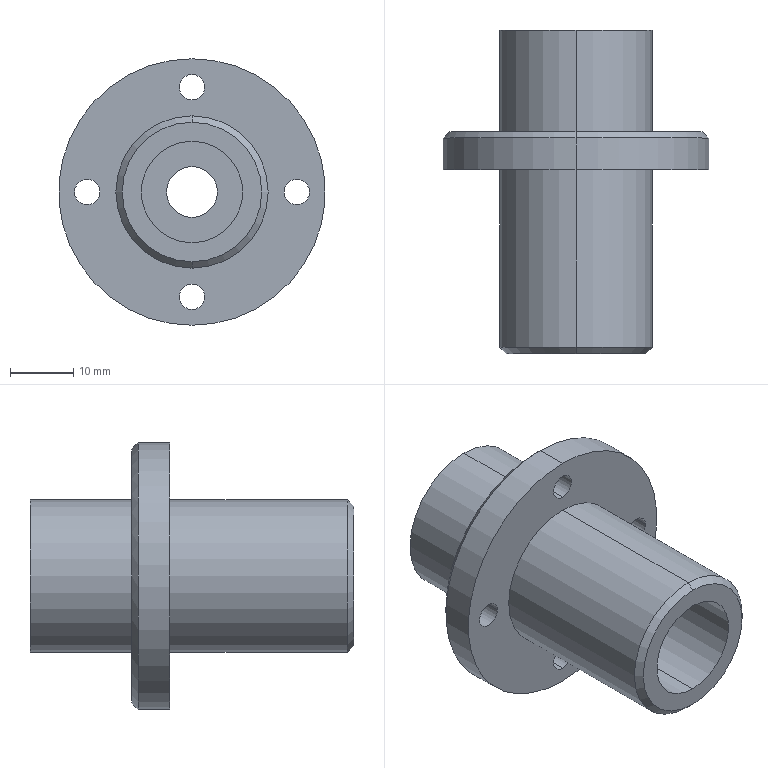Part | SolidWorks | features ICE 4, Chamfer 1, CirPattern 1, Extrusion 1 | 1 solid | 39 faces | box 42 x 51 x 42 mm | volume 18428 mm3 | cylinder 26 | plane 9 | cone 4 | commonest cylinder face diameters 4 x8 6 x8 24 x4 8 x2 16 x2 42 x2
STEP:
#1=CARTESIAN_POINT('',(0.,35.,20.));
#2=VERTEX_POINT('',#1);
#3=CARTESIAN_POINT('',(0.,35.,-20.));
#4=VERTEX_POINT('',#3);
#5=CARTESIAN_POINT('',(0.,35.,0.));
#6=DIRECTION('',(0.,1.,0.));
#7=DIRECTION('',(0.,0.,1.));
#8=AXIS2_PLACEMENT_3D('',#5,#6,#7);
#9=CIRCLE('',#8,20.);
#10=EDGE_CURVE('',#2,#4,#9,.T.);
#11=ORIENTED_EDGE('',*,*,#10,.F.);
#12=CARTESIAN_POINT('',(0.,34.,21.));
#13=VERTEX_POINT('',#12);
#14=CARTESIAN_POINT('',(0.,35.,20.));
#15=DIRECTION('',(0.,-0.7071,0.7071));
#16=VECTOR('',#15,1000.);
#17=LINE('',#14,#16);
#18=EDGE_CURVE('',#2,#13,#17,.T.);
#19=ORIENTED_EDGE('',*,*,#18,.T.);
#20=CARTESIAN_POINT('',(0.,34.,-21.));
#21=VERTEX_POINT('',#20);
#22=CARTESIAN_POINT('',(0.,34.,0.));
#23=DIRECTION('',(0.,-1.,0.));
#24=DIRECTION('',(0.,0.,1.));
#25=AXIS2_PLACEMENT_3D('',#22,#23,#24);
#26=CIRCLE('',#25,21.);
#27=EDGE_CURVE('',#21,#13,#26,.T.);
#28=ORIENTED_EDGE('',*,*,#27,.F.);
#29=CARTESIAN_POINT('',(0.,35.,-20.));
#30=DIRECTION('',(0.,-0.7071,-0.7071));
#31=VECTOR('',#30,1000.);
#32=LINE('',#29,#31);
#33=EDGE_CURVE('',#4,#21,#32,.T.);
#34=ORIENTED_EDGE('',*,*,#33,.F.);
#35=EDGE_LOOP('',(#11,#19,#28,#34));
#36=FACE_OUTER_BOUND('',#35,.T.);
#37=CARTESIAN_POINT('',(0.,35.,0.));
#38=DIRECTION('',(0.,-1.,0.));
#39=DIRECTION('',(0.,0.,-1.));
#40=AXIS2_PLACEMENT_3D('',#37,#38,#39);
#41=CONICAL_SURFACE('',#40,20.,0.7854);
#42=ADVANCED_FACE('',(#36),#41,.T.);
#43=CARTESIAN_POINT('',(0.,0.,-11.));
#44=VERTEX_POINT('',#43);
#45=CARTESIAN_POINT('',(0.,0.,11.));
#46=VERTEX_POINT('',#45);
#47=CARTESIAN_POINT('',(0.,0.,0.));
#48=DIRECTION('',(0.,-1.,0.));
#49=DIRECTION('',(0.,0.,1.));
#50=AXIS2_PLACEMENT_3D('',#47,#48,#49);
#51=CIRCLE('',#50,11.);
#52=EDGE_CURVE('',#44,#46,#51,.T.);
#53=ORIENTED_EDGE('',*,*,#52,.F.);
#54=CARTESIAN_POINT('',(0.,1.,-12.));
#55=VERTEX_POINT('',#54);
#56=CARTESIAN_POINT('',(0.,1.,-12.));
#57=DIRECTION('',(0.,0.7071,-0.7071));
#58=VECTOR('',#57,1000.);
#59=LINE('',#56,#58);
#60=EDGE_CURVE('',#44,#55,#59,.T.);
#61=ORIENTED_EDGE('',*,*,#60,.T.);
#62=CARTESIAN_POINT('',(0.,1.,12.));
#63=VERTEX_POINT('',#62);
#64=CARTESIAN_POINT('',(0.,1.,0.));
#65=DIRECTION('',(0.,1.,0.));
#66=DIRECTION('',(0.,0.,1.));
#67=AXIS2_PLACEMENT_3D('',#64,#65,#66);
#68=CIRCLE('',#67,12.);
#69=EDGE_CURVE('',#63,#55,#68,.T.);
#70=ORIENTED_EDGE('',*,*,#69,.F.);
#71=CARTESIAN_POINT('',(0.,1.,12.));
#72=DIRECTION('',(0.,0.7071,0.7071));
#73=VECTOR('',#72,1000.);
#74=LINE('',#71,#73);
#75=EDGE_CURVE('',#46,#63,#74,.T.);
#76=ORIENTED_EDGE('',*,*,#75,.F.);
#77=EDGE_LOOP('',(#53,#61,#70,#76));
#78=FACE_OUTER_BOUND('',#77,.T.);
#79=CARTESIAN_POINT('',(0.,1.,0.));
#80=DIRECTION('',(0.,1.,0.));
#81=DIRECTION('',(0.,0.,1.));
#82=AXIS2_PLACEMENT_3D('',#79,#80,#81);
#83=CONICAL_SURFACE('',#82,12.,0.7854);
#84=ADVANCED_FACE('',(#78),#83,.T.);
#85=CARTESIAN_POINT('',(-19.5,32.,0.));
#86=VERTEX_POINT('',#85);
#87=CARTESIAN_POINT('',(-13.5,32.,0.));
#88=VERTEX_POINT('',#87);
#89=CARTESIAN_POINT('',(-16.5,32.,0.));
#90=DIRECTION('',(0.,1.,0.));
#91=DIRECTION('',(1.,0.,0.));
#92=AXIS2_PLACEMENT_3D('',#89,#90,#91);
#93=CIRCLE('',#92,3.);
#94=EDGE_CURVE('',#86,#88,#93,.T.);
#95=ORIENTED_EDGE('',*,*,#94,.F.);
#96=CARTESIAN_POINT('',(-19.5,35.,0.));
#97=VERTEX_POINT('',#96);
#98=CARTESIAN_POINT('',(-19.5,32.,0.));
#99=DIRECTION('',(0.,1.,0.));
#100=VECTOR('',#99,1000.);
#101=LINE('',#98,#100);
#102=EDGE_CURVE('',#86,#97,#101,.T.);
#103=ORIENTED_EDGE('',*,*,#102,.T.);
#104=CARTESIAN_POINT('',(-13.5,35.,0.));
#105=VERTEX_POINT('',#104);
#106=CARTESIAN_POINT('',(-16.5,35.,0.));
#107=DIRECTION('',(0.,1.,0.));
#108=DIRECTION('',(1.,0.,0.));
#109=AXIS2_PLACEMENT_3D('',#106,#107,#108);
#110=CIRCLE('',#109,3.);
#111=EDGE_CURVE('',#97,#105,#110,.T.);
#112=ORIENTED_EDGE('',*,*,#111,.T.);
#113=CARTESIAN_POINT('',(-13.5,32.,0.));
#114=DIRECTION('',(0.,1.,0.));
#115=VECTOR('',#114,1000.);
#116=LINE('',#113,#115);
#117=EDGE_CURVE('',#88,#105,#116,.T.);
#118=ORIENTED_EDGE('',*,*,#117,.F.);
#119=EDGE_LOOP('',(#95,#103,#112,#118));
#120=FACE_OUTER_BOUND('',#119,.T.);
#121=CARTESIAN_POINT('',(-16.5,32.,0.));
#122=DIRECTION('',(0.,1.,0.));
#123=DIRECTION('',(1.,0.,0.));
#124=AXIS2_PLACEMENT_3D('',#121,#122,#123);
#125=CYLINDRICAL_SURFACE('',#124,3.);
#126=ADVANCED_FACE('',(#120),#125,.F.);
#127=CARTESIAN_POINT('',(0.,32.,19.5));
#128=VERTEX_POINT('',#127);
#129=CARTESIAN_POINT('',(0.,32.,13.5));
#130=VERTEX_POINT('',#129);
#131=CARTESIAN_POINT('',(0.,32.,16.5));
#132=DIRECTION('',(0.,1.,0.));
#133=DIRECTION('',(0.,0.,-1.));
#134=AXIS2_PLACEMENT_3D('',#131,#132,#133);
#135=CIRCLE('',#134,3.);
#136=EDGE_CURVE('',#128,#130,#135,.T.);
#137=ORIENTED_EDGE('',*,*,#136,.F.);
#138=CARTESIAN_POINT('',(0.,35.,19.5));
#139=VERTEX_POINT('',#138);
#140=CARTESIAN_POINT('',(0.,32.,19.5));
#141=DIRECTION('',(0.,1.,0.));
#142=VECTOR('',#141,1000.);
#143=LINE('',#140,#142);
#144=EDGE_CURVE('',#128,#139,#143,.T.);
#145=ORIENTED_EDGE('',*,*,#144,.T.);
#146=CARTESIAN_POINT('',(0.,35.,13.5));
#147=VERTEX_POINT('',#146);
#148=CARTESIAN_POINT('',(0.,35.,16.5));
#149=DIRECTION('',(0.,1.,0.));
#150=DIRECTION('',(0.,0.,-1.));
#151=AXIS2_PLACEMENT_3D('',#148,#149,#150);
#152=CIRCLE('',#151,3.);
#153=EDGE_CURVE('',#139,#147,#152,.T.);
#154=ORIENTED_EDGE('',*,*,#153,.T.);
#155=CARTESIAN_POINT('',(0.,32.,13.5));
#156=DIRECTION('',(0.,1.,0.));
#157=VECTOR('',#156,1000.);
#158=LINE('',#155,#157);
#159=EDGE_CURVE('',#130,#147,#158,.T.);
#160=ORIENTED_EDGE('',*,*,#159,.F.);
#161=EDGE_LOOP('',(#137,#145,#154,#160));
#162=FACE_OUTER_BOUND('',#161,.T.);
#163=CARTESIAN_POINT('',(0.,32.,16.5));
#164=DIRECTION('',(0.,1.,0.));
#165=DIRECTION('',(0.,0.,-1.));
#166=AXIS2_PLACEMENT_3D('',#163,#164,#165);
#167=CYLINDRICAL_SURFACE('',#166,3.);
#168=ADVANCED_FACE('',(#162),#167,.F.);
#169=CARTESIAN_POINT('',(19.5,32.,0.));
#170=VERTEX_POINT('',#169);
#171=CARTESIAN_POINT('',(13.5,32.,0.));
#172=VERTEX_POINT('',#171);
#173=CARTESIAN_POINT('',(16.5,32.,0.));
#174=DIRECTION('',(0.,1.,0.));
#175=DIRECTION('',(-1.,0.,0.));
#176=AXIS2_PLACEMENT_3D('',#173,#174,#175);
#177=CIRCLE('',#176,3.);
#178=EDGE_CURVE('',#170,#172,#177,.T.);
#179=ORIENTED_EDGE('',*,*,#178,.F.);
#180=CARTESIAN_POINT('',(19.5,35.,0.));
#181=VERTEX_POINT('',#180);
#182=CARTESIAN_POINT('',(19.5,32.,0.));
#183=DIRECTION('',(0.,1.,0.));
#184=VECTOR('',#183,1000.);
#185=LINE('',#182,#184);
#186=EDGE_CURVE('',#170,#181,#185,.T.);
#187=ORIENTED_EDGE('',*,*,#186,.T.);
#188=CARTESIAN_POINT('',(13.5,35.,0.));
#189=VERTEX_POINT('',#188);
#190=CARTESIAN_POINT('',(16.5,35.,0.));
#191=DIRECTION('',(0.,1.,0.));
#192=DIRECTION('',(-1.,0.,0.));
#193=AXIS2_PLACEMENT_3D('',#190,#191,#192);
#194=CIRCLE('',#193,3.);
#195=EDGE_CURVE('',#181,#189,#194,.T.);
#196=ORIENTED_EDGE('',*,*,#195,.T.);
#197=CARTESIAN_POINT('',(13.5,32.,0.));
#198=DIRECTION('',(0.,1.,0.));
#199=VECTOR('',#198,1000.);
#200=LINE('',#197,#199);
#201=EDGE_CURVE('',#172,#189,#200,.T.);
#202=ORIENTED_EDGE('',*,*,#201,.F.);
#203=EDGE_LOOP('',(#179,#187,#196,#202));
#204=FACE_OUTER_BOUND('',#203,.T.);
#205=CARTESIAN_POINT('',(16.5,32.,0.));
#206=DIRECTION('',(0.,1.,0.));
#207=DIRECTION('',(-1.,0.,0.));
#208=AXIS2_PLACEMENT_3D('',#205,#206,#207);
#209=CYLINDRICAL_SURFACE('',#208,3.);
#210=ADVANCED_FACE('',(#204),#209,.F.);
#211=CARTESIAN_POINT('',(-18.5,29.,0.));
#212=VERTEX_POINT('',#211);
#213=CARTESIAN_POINT('',(-14.5,29.,0.));
#214=VERTEX_POINT('',#213);
#215=CARTESIAN_POINT('',(-16.5,29.,0.));
#216=DIRECTION('',(0.,1.,0.));
#217=DIRECTION('',(1.,0.,0.));
#218=AXIS2_PLACEMENT_3D('',#215,#216,#217);
#219=CIRCLE('',#218,2.);
#220=EDGE_CURVE('',#212,#214,#219,.T.);
#221=ORIENTED_EDGE('',*,*,#220,.F.);
#222=CARTESIAN_POINT('',(-18.5,32.,0.));
#223=VERTEX_POINT('',#222);
#224=CARTESIAN_POINT('',(-18.5,29.,0.));
#225=DIRECTION('',(0.,1.,0.));
#226=VECTOR('',#225,1000.);
#227=LINE('',#224,#226);
#228=EDGE_CURVE('',#212,#223,#227,.T.);
#229=ORIENTED_EDGE('',*,*,#228,.T.);
#230=CARTESIAN_POINT('',(-14.5,32.,0.));
#231=VERTEX_POINT('',#230);
#232=CARTESIAN_POINT('',(-16.5,32.,0.));
#233=DIRECTION('',(0.,-1.,0.));
#234=DIRECTION('',(0.,0.,1.));
#235=AXIS2_PLACEMENT_3D('',#232,#233,#234);
#236=CIRCLE('',#235,2.);
#237=EDGE_CURVE('',#231,#223,#236,.T.);
#238=ORIENTED_EDGE('',*,*,#237,.F.);
#239=CARTESIAN_POINT('',(-14.5,29.,0.));
#240=DIRECTION('',(0.,1.,0.));
#241=VECTOR('',#240,1000.);
#242=LINE('',#239,#241);
#243=EDGE_CURVE('',#214,#231,#242,.T.);
#244=ORIENTED_EDGE('',*,*,#243,.F.);
#245=EDGE_LOOP('',(#221,#229,#238,#244));
#246=FACE_OUTER_BOUND('',#245,.T.);
#247=CARTESIAN_POINT('',(-16.5,29.,0.));
#248=DIRECTION('',(0.,1.,0.));
#249=DIRECTION('',(1.,0.,0.));
#250=AXIS2_PLACEMENT_3D('',#247,#248,#249);
#251=CYLINDRICAL_SURFACE('',#250,2.);
#252=ADVANCED_FACE('',(#246),#251,.F.);
#253=CARTESIAN_POINT('',(0.,29.,18.5));
#254=VERTEX_POINT('',#253);
#255=CARTESIAN_POINT('',(0.,29.,14.5));
#256=VERTEX_POINT('',#255);
#257=CARTESIAN_POINT('',(0.,29.,16.5));
#258=DIRECTION('',(0.,1.,0.));
#259=DIRECTION('',(0.,0.,-1.));
#260=AXIS2_PLACEMENT_3D('',#257,#258,#259);
#261=CIRCLE('',#260,2.);
#262=EDGE_CURVE('',#254,#256,#261,.T.);
#263=ORIENTED_EDGE('',*,*,#262,.F.);
#264=CARTESIAN_POINT('',(0.,32.,18.5));
#265=VERTEX_POINT('',#264);
#266=CARTESIAN_POINT('',(0.,29.,18.5));
#267=DIRECTION('',(0.,1.,0.));
#268=VECTOR('',#267,1000.);
#269=LINE('',#266,#268);
#270=EDGE_CURVE('',#254,#265,#269,.T.);
#271=ORIENTED_EDGE('',*,*,#270,.T.);
#272=CARTESIAN_POINT('',(0.,32.,14.5));
#273=VERTEX_POINT('',#272);
#274=CARTESIAN_POINT('',(0.,32.,16.5));
#275=DIRECTION('',(0.,-1.,0.));
#276=DIRECTION('',(0.,0.,1.));
#277=AXIS2_PLACEMENT_3D('',#274,#275,#276);
#278=CIRCLE('',#277,2.);
#279=EDGE_CURVE('',#273,#265,#278,.T.);
#280=ORIENTED_EDGE('',*,*,#279,.F.);
#281=CARTESIAN_POINT('',(0.,29.,14.5));
#282=DIRECTION('',(0.,1.,0.));
#283=VECTOR('',#282,1000.);
#284=LINE('',#281,#283);
#285=EDGE_CURVE('',#256,#273,#284,.T.);
#286=ORIENTED_EDGE('',*,*,#285,.F.);
#287=EDGE_LOOP('',(#263,#271,#280,#286));
#288=FACE_OUTER_BOUND('',#287,.T.);
#289=CARTESIAN_POINT('',(0.,29.,16.5));
#290=DIRECTION('',(0.,1.,0.));
#291=DIRECTION('',(0.,0.,-1.));
#292=AXIS2_PLACEMENT_3D('',#289,#290,#291);
#293=CYLINDRICAL_SURFACE('',#292,2.);
#294=ADVANCED_FACE('',(#288),#293,.F.);
#295=CARTESIAN_POINT('',(18.5,29.,0.));
#296=VERTEX_POINT('',#295);
#297=CARTESIAN_POINT('',(14.5,29.,0.));
#298=VERTEX_POINT('',#297);
#299=CARTESIAN_POINT('',(16.5,29.,0.));
#300=DIRECTION('',(0.,1.,0.));
#301=DIRECTION('',(-1.,0.,0.));
#302=AXIS2_PLACEMENT_3D('',#299,#300,#301);
#303=CIRCLE('',#302,2.);
#304=EDGE_CURVE('',#296,#298,#303,.T.);
#305=ORIENTED_EDGE('',*,*,#304,.F.);
#306=CARTESIAN_POINT('',(18.5,32.,0.));
#307=VERTEX_POINT('',#306);
#308=CARTESIAN_POINT('',(18.5,29.,0.));
#309=DIRECTION('',(0.,1.,0.));
#310=VECTOR('',#309,1000.);
#311=LINE('',#308,#310);
#312=EDGE_CURVE('',#296,#307,#311,.T.);
#313=ORIENTED_EDGE('',*,*,#312,.T.);
#314=CARTESIAN_POINT('',(14.5,32.,0.));
#315=VERTEX_POINT('',#314);
#316=CARTESIAN_POINT('',(16.5,32.,0.));
#317=DIRECTION('',(0.,-1.,0.));
#318=DIRECTION('',(0.,0.,1.));
#319=AXIS2_PLACEMENT_3D('',#316,#317,#318);
#320=CIRCLE('',#319,2.);
#321=EDGE_CURVE('',#315,#307,#320,.T.);
#322=ORIENTED_EDGE('',*,*,#321,.F.);
#323=CARTESIAN_POINT('',(14.5,29.,0.));
#324=DIRECTION('',(0.,1.,0.));
#325=VECTOR('',#324,1000.);
#326=LINE('',#323,#325);
#327=EDGE_CURVE('',#298,#315,#326,.T.);
#328=ORIENTED_EDGE('',*,*,#327,.F.);
#329=EDGE_LOOP('',(#305,#313,#322,#328));
#330=FACE_OUTER_BOUND('',#329,.T.);
#331=CARTESIAN_POINT('',(16.5,29.,0.));
#332=DIRECTION('',(0.,1.,0.));
#333=DIRECTION('',(-1.,0.,0.));
#334=AXIS2_PLACEMENT_3D('',#331,#332,#333);
#335=CYLINDRICAL_SURFACE('',#334,2.);
#336=ADVANCED_FACE('',(#330),#335,.F.);
#337=CARTESIAN_POINT('',(0.,32.,-19.5));
#338=VERTEX_POINT('',#337);
#339=CARTESIAN_POINT('',(0.,32.,-13.5));
#340=VERTEX_POINT('',#339);
#341=CARTESIAN_POINT('',(0.,32.,-16.5));
#342=DIRECTION('',(0.,1.,0.));
#343=DIRECTION('',(0.,0.,1.));
#344=AXIS2_PLACEMENT_3D('',#341,#342,#343);
#345=CIRCLE('',#344,3.);
#346=EDGE_CURVE('',#338,#340,#345,.T.);
#347=ORIENTED_EDGE('',*,*,#346,.F.);
#348=CARTESIAN_POINT('',(0.,35.,-19.5));
#349=VERTEX_POINT('',#348);
#350=CARTESIAN_POINT('',(0.,32.,-19.5));
#351=DIRECTION('',(0.,1.,0.));
#352=VECTOR('',#351,1000.);
#353=LINE('',#350,#352);
#354=EDGE_CURVE('',#338,#349,#353,.T.);
#355=ORIENTED_EDGE('',*,*,#354,.T.);
#356=CARTESIAN_POINT('',(0.,35.,-13.5));
#357=VERTEX_POINT('',#356);
#358=CARTESIAN_POINT('',(0.,35.,-16.5));
#359=DIRECTION('',(0.,1.,0.));
#360=DIRECTION('',(0.,0.,1.));
#361=AXIS2_PLACEMENT_3D('',#358,#359,#360);
#362=CIRCLE('',#361,3.);
#363=EDGE_CURVE('',#349,#357,#362,.T.);
#364=ORIENTED_EDGE('',*,*,#363,.T.);
#365=CARTESIAN_POINT('',(0.,32.,-13.5));
#366=DIRECTION('',(0.,1.,0.));
#367=VECTOR('',#366,1000.);
#368=LINE('',#365,#367);
#369=EDGE_CURVE('',#340,#357,#368,.T.);
#370=ORIENTED_EDGE('',*,*,#369,.F.);
#371=EDGE_LOOP('',(#347,#355,#364,#370));
#372=FACE_OUTER_BOUND('',#371,.T.);
#373=CARTESIAN_POINT('',(0.,32.,-16.5));
#374=DIRECTION('',(0.,1.,0.));
#375=DIRECTION('',(0.,0.,1.));
#376=AXIS2_PLACEMENT_3D('',#373,#374,#375);
#377=CYLINDRICAL_SURFACE('',#376,3.);
#378=ADVANCED_FACE('',(#372),#377,.F.);
#379=CARTESIAN_POINT('',(0.,29.,21.));
#380=VERTEX_POINT('',#379);
#381=CARTESIAN_POINT('',(0.,29.,-21.));
#382=VERTEX_POINT('',#381);
#383=CARTESIAN_POINT('',(0.,29.,0.));
#384=DIRECTION('',(0.,1.,0.));
#385=DIRECTION('',(0.,0.,1.));
#386=AXIS2_PLACEMENT_3D('',#383,#384,#385);
#387=CIRCLE('',#386,21.);
#388=EDGE_CURVE('',#380,#382,#387,.T.);
#389=ORIENTED_EDGE('',*,*,#388,.T.);
#390=CARTESIAN_POINT('',(0.,29.,-21.));
#391=DIRECTION('',(0.,1.,0.));
#392=VECTOR('',#391,1000.);
#393=LINE('',#390,#392);
#394=EDGE_CURVE('',#382,#21,#393,.T.);
#395=ORIENTED_EDGE('',*,*,#394,.T.);
#396=ORIENTED_EDGE('',*,*,#27,.T.);
#397=CARTESIAN_POINT('',(0.,29.,21.));
#398=DIRECTION('',(0.,1.,0.));
#399=VECTOR('',#398,1000.);
#400=LINE('',#397,#399);
#401=EDGE_CURVE('',#380,#13,#400,.T.);
#402=ORIENTED_EDGE('',*,*,#401,.F.);
#403=EDGE_LOOP('',(#389,#395,#396,#402));
#404=FACE_OUTER_BOUND('',#403,.T.);
#405=CARTESIAN_POINT('',(0.,29.,0.));
#406=DIRECTION('',(0.,1.,0.));
#407=DIRECTION('',(0.,0.,1.));
#408=AXIS2_PLACEMENT_3D('',#405,#406,#407);
#409=CYLINDRICAL_SURFACE('',#408,21.);
#410=ADVANCED_FACE('',(#404),#409,.T.);
#411=CARTESIAN_POINT('',(0.,47.,8.));
#412=VERTEX_POINT('',#411);
#413=CARTESIAN_POINT('',(0.,47.,-8.));
#414=VERTEX_POINT('',#413);
#415=CARTESIAN_POINT('',(0.,47.,0.));
#416=DIRECTION('',(0.,-1.,0.));
#417=DIRECTION('',(0.,0.,-1.));
#418=AXIS2_PLACEMENT_3D('',#415,#416,#417);
#419=CIRCLE('',#418,8.);
#420=EDGE_CURVE('',#412,#414,#419,.T.);
#421=ORIENTED_EDGE('',*,*,#420,.F.);
#422=CARTESIAN_POINT('',(0.,0.,8.));
#423=VERTEX_POINT('',#422);
#424=CARTESIAN_POINT('',(0.,47.,8.));
#425=DIRECTION('',(0.,-1.,0.));
#426=VECTOR('',#425,1000.);
#427=LINE('',#424,#426);
#428=EDGE_CURVE('',#412,#423,#427,.T.);
#429=ORIENTED_EDGE('',*,*,#428,.T.);
#430=CARTESIAN_POINT('',(0.,0.,-8.));
#431=VERTEX_POINT('',#430);
#432=CARTESIAN_POINT('',(0.,0.,0.));
#433=DIRECTION('',(0.,-1.,0.));
#434=DIRECTION('',(0.,0.,-1.));
#435=AXIS2_PLACEMENT_3D('',#432,#433,#434);
#436=CIRCLE('',#435,8.);
#437=EDGE_CURVE('',#423,#431,#436,.T.);
#438=ORIENTED_EDGE('',*,*,#437,.T.);
#439=CARTESIAN_POINT('',(0.,47.,-8.));
#440=DIRECTION('',(0.,-1.,0.));
#441=VECTOR('',#440,1000.);
#442=LINE('',#439,#441);
#443=EDGE_CURVE('',#414,#431,#442,.T.);
#444=ORIENTED_EDGE('',*,*,#443,.F.);
#445=EDGE_LOOP('',(#421,#429,#438,#444));
#446=FACE_OUTER_BOUND('',#445,.T.);
#447=CARTESIAN_POINT('',(0.,47.,0.));
#448=DIRECTION('',(0.,-1.,0.));
#449=DIRECTION('',(0.,0.,-1.));
#450=AXIS2_PLACEMENT_3D('',#447,#448,#449);
#451=CYLINDRICAL_SURFACE('',#450,8.);
#452=ADVANCED_FACE('',(#446),#451,.F.);
#453=CARTESIAN_POINT('',(0.,51.,12.));
#454=VERTEX_POINT('',#453);
#455=CARTESIAN_POINT('',(0.,51.,-12.));
#456=VERTEX_POINT('',#455);
#457=CARTESIAN_POINT('',(0.,51.,0.));
#458=DIRECTION('',(0.,1.,0.));
#459=DIRECTION('',(0.,0.,1.));
#460=AXIS2_PLACEMENT_3D('',#457,#458,#459);
#461=CIRCLE('',#460,12.);
#462=EDGE_CURVE('',#454,#456,#461,.T.);
#463=ORIENTED_EDGE('',*,*,#462,.F.);
#464=CARTESIAN_POINT('',(0.,35.,12.));
#465=VERTEX_POINT('',#464);
#466=CARTESIAN_POINT('',(0.,51.,12.));
#467=DIRECTION('',(0.,-1.,0.));
#468=VECTOR('',#467,1000.);
#469=LINE('',#466,#468);
#470=EDGE_CURVE('',#454,#465,#469,.T.);
#471=ORIENTED_EDGE('',*,*,#470,.T.);
#472=CARTESIAN_POINT('',(0.,35.,-12.));
#473=VERTEX_POINT('',#472);
#474=CARTESIAN_POINT('',(0.,35.,0.));
#475=DIRECTION('',(0.,1.,0.));
#476=DIRECTION('',(0.,0.,1.));
#477=AXIS2_PLACEMENT_3D('',#474,#475,#476);
#478=CIRCLE('',#477,12.);
#479=EDGE_CURVE('',#465,#473,#478,.T.);
#480=ORIENTED_EDGE('',*,*,#479,.T.);
#481=CARTESIAN_POINT('',(0.,51.,-12.));
#482=DIRECTION('',(0.,-1.,0.));
#483=VECTOR('',#482,1000.);
#484=LINE('',#481,#483);
#485=EDGE_CURVE('',#456,#473,#484,.T.);
#486=ORIENTED_EDGE('',*,*,#485,.F.);
#487=EDGE_LOOP('',(#463,#471,#480,#486));
#488=FACE_OUTER_BOUND('',#487,.T.);
#489=CARTESIAN_POINT('',(0.,51.,0.));
#490=DIRECTION('',(0.,-1.,0.));
#491=DIRECTION('',(0.,0.,-1.));
#492=AXIS2_PLACEMENT_3D('',#489,#490,#491);
#493=CYLINDRICAL_SURFACE('',#492,12.);
#494=ADVANCED_FACE('',(#488),#493,.T.);
#495=CARTESIAN_POINT('',(0.,51.,-4.));
#496=VERTEX_POINT('',#495);
#497=CARTESIAN_POINT('',(0.,51.,4.));
#498=VERTEX_POINT('',#497);
#499=CARTESIAN_POINT('',(0.,51.,0.));
#500=DIRECTION('',(0.,1.,0.));
#501=DIRECTION('',(0.,0.,1.));
#502=AXIS2_PLACEMENT_3D('',#499,#500,#501);
#503=CIRCLE('',#502,4.);
#504=EDGE_CURVE('',#496,#498,#503,.T.);
#505=ORIENTED_EDGE('',*,*,#504,.T.);
#506=CARTESIAN_POINT('',(0.,47.,4.));
#507=VERTEX_POINT('',#506);
#508=CARTESIAN_POINT('',(0.,51.,4.));
#509=DIRECTION('',(0.,-1.,0.));
#510=VECTOR('',#509,1000.);
#511=LINE('',#508,#510);
#512=EDGE_CURVE('',#498,#507,#511,.T.);
#513=ORIENTED_EDGE('',*,*,#512,.T.);
#514=CARTESIAN_POINT('',(0.,47.,-4.));
#515=VERTEX_POINT('',#514);
#516=CARTESIAN_POINT('',(0.,47.,0.));
#517=DIRECTION('',(0.,-1.,0.));
#518=DIRECTION('',(0.,0.,-1.));
#519=AXIS2_PLACEMENT_3D('',#516,#517,#518);
#520=CIRCLE('',#519,4.);
#521=EDGE_CURVE('',#507,#515,#520,.T.);
#522=ORIENTED_EDGE('',*,*,#521,.T.);
#523=CARTESIAN_POINT('',(0.,51.,-4.));
#524=DIRECTION('',(0.,-1.,0.));
#525=VECTOR('',#524,1000.);
#526=LINE('',#523,#525);
#527=EDGE_CURVE('',#496,#515,#526,.T.);
#528=ORIENTED_EDGE('',*,*,#527,.F.);
#529=EDGE_LOOP('',(#505,#513,#522,#528));
#530=FACE_OUTER_BOUND('',#529,.T.);
#531=CARTESIAN_POINT('',(0.,51.,0.));
#532=DIRECTION('',(0.,-1.,0.));
#533=DIRECTION('',(0.,0.,-1.));
#534=AXIS2_PLACEMENT_3D('',#531,#532,#533);
#535=CYLINDRICAL_SURFACE('',#534,4.);
#536=ADVANCED_FACE('',(#530),#535,.F.);
#537=CARTESIAN_POINT('',(0.,29.,12.));
#538=VERTEX_POINT('',#537);
#539=CARTESIAN_POINT('',(0.,29.,-12.));
#540=VERTEX_POINT('',#539);
#541=CARTESIAN_POINT('',(0.,29.,0.));
#542=DIRECTION('',(0.,1.,0.));
#543=DIRECTION('',(0.,0.,1.));
#544=AXIS2_PLACEMENT_3D('',#541,#542,#543);
#545=CIRCLE('',#544,12.);
#546=EDGE_CURVE('',#538,#540,#545,.T.);
#547=ORIENTED_EDGE('',*,*,#546,.F.);
#548=CARTESIAN_POINT('',(0.,51.,12.));
#549=DIRECTION('',(0.,-1.,0.));
#550=VECTOR('',#549,1000.);
#551=LINE('',#548,#550);
#552=EDGE_CURVE('',#538,#63,#551,.T.);
#553=ORIENTED_EDGE('',*,*,#552,.T.);
#554=ORIENTED_EDGE('',*,*,#69,.T.);
#555=CARTESIAN_POINT('',(0.,51.,-12.));
#556=DIRECTION('',(0.,-1.,0.));
#557=VECTOR('',#556,1000.);
#558=LINE('',#555,#557);
#559=EDGE_CURVE('',#540,#55,#558,.T.);
#560=ORIENTED_EDGE('',*,*,#559,.F.);
#561=EDGE_LOOP('',(#547,#553,#554,#560));
#562=FACE_OUTER_BOUND('',#561,.T.);
#563=CARTESIAN_POINT('',(0.,51.,0.));
#564=DIRECTION('',(0.,-1.,0.));
#565=DIRECTION('',(0.,0.,-1.));
#566=AXIS2_PLACEMENT_3D('',#563,#564,#565);
#567=CYLINDRICAL_SURFACE('',#566,12.);
#568=ADVANCED_FACE('',(#562),#567,.T.);
#569=CARTESIAN_POINT('',(0.,29.,-18.5));
#570=VERTEX_POINT('',#569);
#571=CARTESIAN_POINT('',(0.,29.,-14.5));
#572=VERTEX_POINT('',#571);
#573=CARTESIAN_POINT('',(0.,29.,-16.5));
#574=DIRECTION('',(0.,1.,0.));
#575=DIRECTION('',(0.,0.,1.));
#576=AXIS2_PLACEMENT_3D('',#573,#574,#575);
#577=CIRCLE('',#576,2.);
#578=EDGE_CURVE('',#570,#572,#577,.T.);
#579=ORIENTED_EDGE('',*,*,#578,.F.);
#580=CARTESIAN_POINT('',(0.,32.,-18.5));
#581=VERTEX_POINT('',#580);
#582=CARTESIAN_POINT('',(0.,29.,-18.5));
#583=DIRECTION('',(0.,1.,0.));
#584=VECTOR('',#583,1000.);
#585=LINE('',#582,#584);
#586=EDGE_CURVE('',#570,#581,#585,.T.);
#587=ORIENTED_EDGE('',*,*,#586,.T.);
#588=CARTESIAN_POINT('',(0.,32.,-14.5));
#589=VERTEX_POINT('',#588);
#590=CARTESIAN_POINT('',(0.,32.,-16.5));
#591=DIRECTION('',(0.,-1.,0.));
#592=DIRECTION('',(0.,0.,1.));
#593=AXIS2_PLACEMENT_3D('',#590,#591,#592);
#594=CIRCLE('',#593,2.);
#595=EDGE_CURVE('',#589,#581,#594,.T.);
#596=ORIENTED_EDGE('',*,*,#595,.F.);
#597=CARTESIAN_POINT('',(0.,29.,-14.5));
#598=DIRECTION('',(0.,1.,0.));
#599=VECTOR('',#598,1000.);
#600=LINE('',#597,#599);
#601=EDGE_CURVE('',#572,#589,#600,.T.);
#602=ORIENTED_EDGE('',*,*,#601,.F.);
#603=EDGE_LOOP('',(#579,#587,#596,#602));
#604=FACE_OUTER_BOUND('',#603,.T.);
#605=CARTESIAN_POINT('',(0.,29.,-16.5));
#606=DIRECTION('',(0.,1.,0.));
#607=DIRECTION('',(0.,0.,1.));
#608=AXIS2_PLACEMENT_3D('',#605,#606,#607);
#609=CYLINDRICAL_SURFACE('',#608,2.);
#610=ADVANCED_FACE('',(#604),#609,.F.);
#611=ORIENTED_EDGE('',*,*,#586,.F.);
#612=CARTESIAN_POINT('',(0.,29.,-16.5));
#613=DIRECTION('',(0.,1.,0.));
#614=DIRECTION('',(0.,0.,1.));
#615=AXIS2_PLACEMENT_3D('',#612,#613,#614);
#616=CIRCLE('',#615,2.);
#617=EDGE_CURVE('',#572,#570,#616,.T.);
#618=ORIENTED_EDGE('',*,*,#617,.F.);
#619=ORIENTED_EDGE('',*,*,#601,.T.);
#620=CARTESIAN_POINT('',(0.,32.,-16.5));
#621=DIRECTION('',(0.,-1.,0.));
#622=DIRECTION('',(0.,0.,1.));
#623=AXIS2_PLACEMENT_3D('',#620,#621,#622);
#624=CIRCLE('',#623,2.);
#625=EDGE_CURVE('',#581,#589,#624,.T.);
#626=ORIENTED_EDGE('',*,*,#625,.F.);
#627=EDGE_LOOP('',(#611,#618,#619,#626));
#628=FACE_OUTER_BOUND('',#627,.T.);
#629=CARTESIAN_POINT('',(0.,29.,-16.5));
#630=DIRECTION('',(0.,1.,0.));
#631=DIRECTION('',(0.,0.,1.));
#632=AXIS2_PLACEMENT_3D('',#629,#630,#631);
#633=CYLINDRICAL_SURFACE('',#632,2.);
#634=ADVANCED_FACE('',(#628),#633,.F.);
#635=ORIENTED_EDGE('',*,*,#552,.F.);
#636=CARTESIAN_POINT('',(0.,29.,0.));
#637=DIRECTION('',(0.,1.,0.));
#638=DIRECTION('',(0.,0.,1.));
#639=AXIS2_PLACEMENT_3D('',#636,#637,#638);
#640=CIRCLE('',#639,12.);
#641=EDGE_CURVE('',#540,#538,#640,.T.);
#642=ORIENTED_EDGE('',*,*,#641,.F.);
#643=ORIENTED_EDGE('',*,*,#559,.T.);
#644=CARTESIAN_POINT('',(0.,1.,0.));
#645=DIRECTION('',(0.,1.,0.));
#646=DIRECTION('',(0.,0.,1.));
#647=AXIS2_PLACEMENT_3D('',#644,#645,#646);
#648=CIRCLE('',#647,12.);
#649=EDGE_CURVE('',#55,#63,#648,.T.);
#650=ORIENTED_EDGE('',*,*,#649,.T.);
#651=EDGE_LOOP('',(#635,#642,#643,#650));
#652=FACE_OUTER_BOUND('',#651,.T.);
#653=CARTESIAN_POINT('',(0.,51.,0.));
#654=DIRECTION('',(0.,-1.,0.));
#655=DIRECTION('',(0.,0.,-1.));
#656=AXIS2_PLACEMENT_3D('',#653,#654,#655);
#657=CYLINDRICAL_SURFACE('',#656,12.);
#658=ADVANCED_FACE('',(#652),#657,.T.);
#659=ORIENTED_EDGE('',*,*,#512,.F.);
#660=CARTESIAN_POINT('',(0.,51.,0.));
#661=DIRECTION('',(0.,1.,0.));
#662=DIRECTION('',(0.,0.,1.));
#663=AXIS2_PLACEMENT_3D('',#660,#661,#662);
#664=CIRCLE('',#663,4.);
#665=EDGE_CURVE('',#498,#496,#664,.T.);
#666=ORIENTED_EDGE('',*,*,#665,.T.);
#667=ORIENTED_EDGE('',*,*,#527,.T.);
#668=CARTESIAN_POINT('',(0.,47.,0.));
#669=DIRECTION('',(0.,-1.,0.));
#670=DIRECTION('',(0.,0.,-1.));
#671=AXIS2_PLACEMENT_3D('',#668,#669,#670);
#672=CIRCLE('',#671,4.);
#673=EDGE_CURVE('',#515,#507,#672,.T.);
#674=ORIENTED_EDGE('',*,*,#673,.T.);
#675=EDGE_LOOP('',(#659,#666,#667,#674));
#676=FACE_OUTER_BOUND('',#675,.T.);
#677=CARTESIAN_POINT('',(0.,51.,0.));
#678=DIRECTION('',(0.,-1.,0.));
#679=DIRECTION('',(0.,0.,-1.));
#680=AXIS2_PLACEMENT_3D('',#677,#678,#679);
#681=CYLINDRICAL_SURFACE('',#680,4.);
#682=ADVANCED_FACE('',(#676),#681,.F.);
#683=CARTESIAN_POINT('',(0.,51.,0.));
#684=DIRECTION('',(0.,1.,0.));
#685=DIRECTION('',(0.,0.,1.));
#686=AXIS2_PLACEMENT_3D('',#683,#684,#685);
#687=CIRCLE('',#686,12.);
#688=EDGE_CURVE('',#456,#454,#687,.T.);
#689=ORIENTED_EDGE('',*,*,#688,.T.);
#690=ORIENTED_EDGE('',*,*,#462,.T.);
#691=EDGE_LOOP('',(#689,#690));
#692=FACE_OUTER_BOUND('',#691,.T.);
#693=ORIENTED_EDGE('',*,*,#504,.F.);
#694=ORIENTED_EDGE('',*,*,#665,.F.);
#695=EDGE_LOOP('',(#693,#694));
#696=FACE_BOUND('',#695,.T.);
#697=CARTESIAN_POINT('',(0.,51.,0.));
#698=DIRECTION('',(0.,1.,0.));
#699=DIRECTION('',(0.,0.,1.));
#700=AXIS2_PLACEMENT_3D('',#697,#698,#699);
#701=PLANE('',#700);
#702=ADVANCED_FACE('',(#692,#696),#701,.T.);
#703=CARTESIAN_POINT('',(0.,0.,0.));
#704=DIRECTION('',(0.,-1.,0.));
#705=DIRECTION('',(0.,0.,1.));
#706=AXIS2_PLACEMENT_3D('',#703,#704,#705);
#707=CIRCLE('',#706,11.);
#708=EDGE_CURVE('',#46,#44,#707,.T.);
#709=ORIENTED_EDGE('',*,*,#708,.T.);
#710=ORIENTED_EDGE('',*,*,#52,.T.);
#711=EDGE_LOOP('',(#709,#710));
#712=FACE_OUTER_BOUND('',#711,.T.);
#713=CARTESIAN_POINT('',(0.,0.,0.));
#714=DIRECTION('',(0.,-1.,0.));
#715=DIRECTION('',(0.,0.,-1.));
#716=AXIS2_PLACEMENT_3D('',#713,#714,#715);
#717=CIRCLE('',#716,8.);
#718=EDGE_CURVE('',#431,#423,#717,.T.);
#719=ORIENTED_EDGE('',*,*,#718,.F.);
#720=ORIENTED_EDGE('',*,*,#437,.F.);
#721=EDGE_LOOP('',(#719,#720));
#722=FACE_BOUND('',#721,.T.);
#723=CARTESIAN_POINT('',(0.,0.,0.));
#724=DIRECTION('',(0.,1.,0.));
#725=DIRECTION('',(0.,0.,1.));
#726=AXIS2_PLACEMENT_3D('',#723,#724,#725);
#727=PLANE('',#726);
#728=ADVANCED_FACE('',(#712,#722),#727,.F.);
#729=ORIENTED_EDGE('',*,*,#470,.F.);
#730=ORIENTED_EDGE('',*,*,#688,.F.);
#731=ORIENTED_EDGE('',*,*,#485,.T.);
#732=CARTESIAN_POINT('',(0.,35.,0.));
#733=DIRECTION('',(0.,1.,0.));
#734=DIRECTION('',(0.,0.,1.));
#735=AXIS2_PLACEMENT_3D('',#732,#733,#734);
#736=CIRCLE('',#735,12.);
#737=EDGE_CURVE('',#473,#465,#736,.T.);
#738=ORIENTED_EDGE('',*,*,#737,.T.);
#739=EDGE_LOOP('',(#729,#730,#731,#738));
#740=FACE_OUTER_BOUND('',#739,.T.);
#741=CARTESIAN_POINT('',(0.,51.,0.));
#742=DIRECTION('',(0.,-1.,0.));
#743=DIRECTION('',(0.,0.,-1.));
#744=AXIS2_PLACEMENT_3D('',#741,#742,#743);
#745=CYLINDRICAL_SURFACE('',#744,12.);
#746=ADVANCED_FACE('',(#740),#745,.T.);
#747=ORIENTED_EDGE('',*,*,#428,.F.);
#748=CARTESIAN_POINT('',(0.,47.,0.));
#749=DIRECTION('',(0.,-1.,0.));
#750=DIRECTION('',(0.,0.,-1.));
#751=AXIS2_PLACEMENT_3D('',#748,#749,#750);
#752=CIRCLE('',#751,8.);
#753=EDGE_CURVE('',#414,#412,#752,.T.);
#754=ORIENTED_EDGE('',*,*,#753,.F.);
#755=ORIENTED_EDGE('',*,*,#443,.T.);
#756=ORIENTED_EDGE('',*,*,#718,.T.);
#757=EDGE_LOOP('',(#747,#754,#755,#756));
#758=FACE_OUTER_BOUND('',#757,.T.);
#759=CARTESIAN_POINT('',(0.,47.,0.));
#760=DIRECTION('',(0.,-1.,0.));
#761=DIRECTION('',(0.,0.,-1.));
#762=AXIS2_PLACEMENT_3D('',#759,#760,#761);
#763=CYLINDRICAL_SURFACE('',#762,8.);
#764=ADVANCED_FACE('',(#758),#763,.F.);
#765=ORIENTED_EDGE('',*,*,#673,.F.);
#766=ORIENTED_EDGE('',*,*,#521,.F.);
#767=EDGE_LOOP('',(#765,#766));
#768=FACE_BOUND('',#767,.T.);
#769=ORIENTED_EDGE('',*,*,#753,.T.);
#770=ORIENTED_EDGE('',*,*,#420,.T.);
#771=EDGE_LOOP('',(#769,#770));
#772=FACE_OUTER_BOUND('',#771,.T.);
#773=CARTESIAN_POINT('',(0.,47.,0.));
#774=DIRECTION('',(0.,-1.,0.));
#775=DIRECTION('',(0.,0.,-1.));
#776=AXIS2_PLACEMENT_3D('',#773,#774,#775);
#777=PLANE('',#776);
#778=ADVANCED_FACE('',(#768,#772),#777,.T.);
#779=ORIENTED_EDGE('',*,*,#394,.F.);
#780=CARTESIAN_POINT('',(0.,29.,0.));
#781=DIRECTION('',(0.,1.,0.));
#782=DIRECTION('',(0.,0.,1.));
#783=AXIS2_PLACEMENT_3D('',#780,#781,#782);
#784=CIRCLE('',#783,21.);
#785=EDGE_CURVE('',#382,#380,#784,.T.);
#786=ORIENTED_EDGE('',*,*,#785,.T.);
#787=ORIENTED_EDGE('',*,*,#401,.T.);
#788=CARTESIAN_POINT('',(0.,34.,0.));
#789=DIRECTION('',(0.,-1.,0.));
#790=DIRECTION('',(0.,0.,1.));
#791=AXIS2_PLACEMENT_3D('',#788,#789,#790);
#792=CIRCLE('',#791,21.);
#793=EDGE_CURVE('',#13,#21,#792,.T.);
#794=ORIENTED_EDGE('',*,*,#793,.T.);
#795=EDGE_LOOP('',(#779,#786,#787,#794));
#796=FACE_OUTER_BOUND('',#795,.T.);
#797=CARTESIAN_POINT('',(0.,29.,0.));
#798=DIRECTION('',(0.,1.,0.));
#799=DIRECTION('',(0.,0.,1.));
#800=AXIS2_PLACEMENT_3D('',#797,#798,#799);
#801=CYLINDRICAL_SURFACE('',#800,21.);
#802=ADVANCED_FACE('',(#796),#801,.T.);
#803=CARTESIAN_POINT('',(-16.5,29.,0.));
#804=DIRECTION('',(0.,1.,0.));
#805=DIRECTION('',(1.,0.,0.));
#806=AXIS2_PLACEMENT_3D('',#803,#804,#805);
#807=CIRCLE('',#806,2.);
#808=EDGE_CURVE('',#214,#212,#807,.T.);
#809=ORIENTED_EDGE('',*,*,#808,.T.);
#810=ORIENTED_EDGE('',*,*,#220,.T.);
#811=EDGE_LOOP('',(#809,#810));
#812=FACE_BOUND('',#811,.T.);
#813=CARTESIAN_POINT('',(0.,29.,16.5));
#814=DIRECTION('',(0.,1.,0.));
#815=DIRECTION('',(0.,0.,-1.));
#816=AXIS2_PLACEMENT_3D('',#813,#814,#815);
#817=CIRCLE('',#816,2.);
#818=EDGE_CURVE('',#256,#254,#817,.T.);
#819=ORIENTED_EDGE('',*,*,#818,.T.);
#820=ORIENTED_EDGE('',*,*,#262,.T.);
#821=EDGE_LOOP('',(#819,#820));
#822=FACE_BOUND('',#821,.T.);
#823=CARTESIAN_POINT('',(16.5,29.,0.));
#824=DIRECTION('',(0.,1.,0.));
#825=DIRECTION('',(-1.,0.,0.));
#826=AXIS2_PLACEMENT_3D('',#823,#824,#825);
#827=CIRCLE('',#826,2.);
#828=EDGE_CURVE('',#298,#296,#827,.T.);
#829=ORIENTED_EDGE('',*,*,#828,.T.);
#830=ORIENTED_EDGE('',*,*,#304,.T.);
#831=EDGE_LOOP('',(#829,#830));
#832=FACE_BOUND('',#831,.T.);
#833=ORIENTED_EDGE('',*,*,#617,.T.);
#834=ORIENTED_EDGE('',*,*,#578,.T.);
#835=EDGE_LOOP('',(#833,#834));
#836=FACE_BOUND('',#835,.T.);
#837=ORIENTED_EDGE('',*,*,#641,.T.);
#838=ORIENTED_EDGE('',*,*,#546,.T.);
#839=EDGE_LOOP('',(#837,#838));
#840=FACE_BOUND('',#839,.T.);
#841=ORIENTED_EDGE('',*,*,#388,.F.);
#842=ORIENTED_EDGE('',*,*,#785,.F.);
#843=EDGE_LOOP('',(#841,#842));
#844=FACE_OUTER_BOUND('',#843,.T.);
#845=CARTESIAN_POINT('',(0.,29.,0.));
#846=DIRECTION('',(0.,1.,0.));
#847=DIRECTION('',(0.,0.,1.));
#848=AXIS2_PLACEMENT_3D('',#845,#846,#847);
#849=PLANE('',#848);
#850=ADVANCED_FACE('',(#812,#822,#832,#836,#840,#844),#849,.F.);
#851=CARTESIAN_POINT('',(0.,35.,0.));
#852=DIRECTION('',(0.,1.,0.));
#853=DIRECTION('',(0.,0.,1.));
#854=AXIS2_PLACEMENT_3D('',#851,#852,#853);
#855=CIRCLE('',#854,20.);
#856=EDGE_CURVE('',#4,#2,#855,.T.);
#857=ORIENTED_EDGE('',*,*,#856,.T.);
#858=ORIENTED_EDGE('',*,*,#10,.T.);
#859=EDGE_LOOP('',(#857,#858));
#860=FACE_OUTER_BOUND('',#859,.T.);
#861=CARTESIAN_POINT('',(-16.5,35.,0.));
#862=DIRECTION('',(0.,1.,0.));
#863=DIRECTION('',(1.,0.,0.));
#864=AXIS2_PLACEMENT_3D('',#861,#862,#863);
#865=CIRCLE('',#864,3.);
#866=EDGE_CURVE('',#105,#97,#865,.T.);
#867=ORIENTED_EDGE('',*,*,#866,.F.);
#868=ORIENTED_EDGE('',*,*,#111,.F.);
#869=EDGE_LOOP('',(#867,#868));
#870=FACE_BOUND('',#869,.T.);
#871=CARTESIAN_POINT('',(0.,35.,16.5));
#872=DIRECTION('',(0.,1.,0.));
#873=DIRECTION('',(0.,0.,-1.));
#874=AXIS2_PLACEMENT_3D('',#871,#872,#873);
#875=CIRCLE('',#874,3.);
#876=EDGE_CURVE('',#147,#139,#875,.T.);
#877=ORIENTED_EDGE('',*,*,#876,.F.);
#878=ORIENTED_EDGE('',*,*,#153,.F.);
#879=EDGE_LOOP('',(#877,#878));
#880=FACE_BOUND('',#879,.T.);
#881=CARTESIAN_POINT('',(16.5,35.,0.));
#882=DIRECTION('',(0.,1.,0.));
#883=DIRECTION('',(-1.,0.,0.));
#884=AXIS2_PLACEMENT_3D('',#881,#882,#883);
#885=CIRCLE('',#884,3.);
#886=EDGE_CURVE('',#189,#181,#885,.T.);
#887=ORIENTED_EDGE('',*,*,#886,.F.);
#888=ORIENTED_EDGE('',*,*,#195,.F.);
#889=EDGE_LOOP('',(#887,#888));
#890=FACE_BOUND('',#889,.T.);
#891=CARTESIAN_POINT('',(0.,35.,-16.5));
#892=DIRECTION('',(0.,1.,0.));
#893=DIRECTION('',(0.,0.,1.));
#894=AXIS2_PLACEMENT_3D('',#891,#892,#893);
#895=CIRCLE('',#894,3.);
#896=EDGE_CURVE('',#357,#349,#895,.T.);
#897=ORIENTED_EDGE('',*,*,#896,.F.);
#898=ORIENTED_EDGE('',*,*,#363,.F.);
#899=EDGE_LOOP('',(#897,#898));
#900=FACE_BOUND('',#899,.T.);
#901=ORIENTED_EDGE('',*,*,#737,.F.);
#902=ORIENTED_EDGE('',*,*,#479,.F.);
#903=EDGE_LOOP('',(#901,#902));
#904=FACE_BOUND('',#903,.T.);
#905=CARTESIAN_POINT('',(0.,35.,0.));
#906=DIRECTION('',(0.,1.,0.));
#907=DIRECTION('',(0.,0.,1.));
#908=AXIS2_PLACEMENT_3D('',#905,#906,#907);
#909=PLANE('',#908);
#910=ADVANCED_FACE('',(#860,#870,#880,#890,#900,#904),#909,.T.);
#911=CARTESIAN_POINT('',(0.,32.,-16.5));
#912=DIRECTION('',(0.,1.,0.));
#913=DIRECTION('',(0.,0.,1.));
#914=AXIS2_PLACEMENT_3D('',#911,#912,#913);
#915=CIRCLE('',#914,3.);
#916=EDGE_CURVE('',#340,#338,#915,.T.);
#917=ORIENTED_EDGE('',*,*,#916,.T.);
#918=ORIENTED_EDGE('',*,*,#346,.T.);
#919=EDGE_LOOP('',(#917,#918));
#920=FACE_OUTER_BOUND('',#919,.T.);
#921=ORIENTED_EDGE('',*,*,#595,.T.);
#922=ORIENTED_EDGE('',*,*,#625,.T.);
#923=EDGE_LOOP('',(#921,#922));
#924=FACE_BOUND('',#923,.T.);
#925=CARTESIAN_POINT('',(0.,32.,-16.5));
#926=DIRECTION('',(0.,1.,0.));
#927=DIRECTION('',(0.,0.,1.));
#928=AXIS2_PLACEMENT_3D('',#925,#926,#927);
#929=PLANE('',#928);
#930=ADVANCED_FACE('',(#920,#924),#929,.T.);
#931=ORIENTED_EDGE('',*,*,#354,.F.);
#932=ORIENTED_EDGE('',*,*,#916,.F.);
#933=ORIENTED_EDGE('',*,*,#369,.T.);
#934=ORIENTED_EDGE('',*,*,#896,.T.);
#935=EDGE_LOOP('',(#931,#932,#933,#934));
#936=FACE_OUTER_BOUND('',#935,.T.);
#937=CARTESIAN_POINT('',(0.,32.,-16.5));
#938=DIRECTION('',(0.,1.,0.));
#939=DIRECTION('',(0.,0.,1.));
#940=AXIS2_PLACEMENT_3D('',#937,#938,#939);
#941=CYLINDRICAL_SURFACE('',#940,3.);
#942=ADVANCED_FACE('',(#936),#941,.F.);
#943=ORIENTED_EDGE('',*,*,#312,.F.);
#944=ORIENTED_EDGE('',*,*,#828,.F.);
#945=ORIENTED_EDGE('',*,*,#327,.T.);
#946=CARTESIAN_POINT('',(16.5,32.,0.));
#947=DIRECTION('',(0.,-1.,0.));
#948=DIRECTION('',(0.,0.,1.));
#949=AXIS2_PLACEMENT_3D('',#946,#947,#948);
#950=CIRCLE('',#949,2.);
#951=EDGE_CURVE('',#307,#315,#950,.T.);
#952=ORIENTED_EDGE('',*,*,#951,.F.);
#953=EDGE_LOOP('',(#943,#944,#945,#952));
#954=FACE_OUTER_BOUND('',#953,.T.);
#955=CARTESIAN_POINT('',(16.5,29.,0.));
#956=DIRECTION('',(0.,1.,0.));
#957=DIRECTION('',(-1.,0.,0.));
#958=AXIS2_PLACEMENT_3D('',#955,#956,#957);
#959=CYLINDRICAL_SURFACE('',#958,2.);
#960=ADVANCED_FACE('',(#954),#959,.F.);
#961=ORIENTED_EDGE('',*,*,#270,.F.);
#962=ORIENTED_EDGE('',*,*,#818,.F.);
#963=ORIENTED_EDGE('',*,*,#285,.T.);
#964=CARTESIAN_POINT('',(0.,32.,16.5));
#965=DIRECTION('',(0.,-1.,0.));
#966=DIRECTION('',(0.,0.,1.));
#967=AXIS2_PLACEMENT_3D('',#964,#965,#966);
#968=CIRCLE('',#967,2.);
#969=EDGE_CURVE('',#265,#273,#968,.T.);
#970=ORIENTED_EDGE('',*,*,#969,.F.);
#971=EDGE_LOOP('',(#961,#962,#963,#970));
#972=FACE_OUTER_BOUND('',#971,.T.);
#973=CARTESIAN_POINT('',(0.,29.,16.5));
#974=DIRECTION('',(0.,1.,0.));
#975=DIRECTION('',(0.,0.,-1.));
#976=AXIS2_PLACEMENT_3D('',#973,#974,#975);
#977=CYLINDRICAL_SURFACE('',#976,2.);
#978=ADVANCED_FACE('',(#972),#977,.F.);
#979=ORIENTED_EDGE('',*,*,#228,.F.);
#980=ORIENTED_EDGE('',*,*,#808,.F.);
#981=ORIENTED_EDGE('',*,*,#243,.T.);
#982=CARTESIAN_POINT('',(-16.5,32.,0.));
#983=DIRECTION('',(0.,-1.,0.));
#984=DIRECTION('',(0.,0.,1.));
#985=AXIS2_PLACEMENT_3D('',#982,#983,#984);
#986=CIRCLE('',#985,2.);
#987=EDGE_CURVE('',#223,#231,#986,.T.);
#988=ORIENTED_EDGE('',*,*,#987,.F.);
#989=EDGE_LOOP('',(#979,#980,#981,#988));
#990=FACE_OUTER_BOUND('',#989,.T.);
#991=CARTESIAN_POINT('',(-16.5,29.,0.));
#992=DIRECTION('',(0.,1.,0.));
#993=DIRECTION('',(1.,0.,0.));
#994=AXIS2_PLACEMENT_3D('',#991,#992,#993);
#995=CYLINDRICAL_SURFACE('',#994,2.);
#996=ADVANCED_FACE('',(#990),#995,.F.);
#997=CARTESIAN_POINT('',(16.5,32.,0.));
#998=DIRECTION('',(0.,1.,0.));
#999=DIRECTION('',(-1.,0.,0.));
#1000=AXIS2_PLACEMENT_3D('',#997,#998,#999);
#1001=CIRCLE('',#1000,3.);
#1002=EDGE_CURVE('',#172,#170,#1001,.T.);
#1003=ORIENTED_EDGE('',*,*,#1002,.T.);
#1004=ORIENTED_EDGE('',*,*,#178,.T.);
#1005=EDGE_LOOP('',(#1003,#1004));
#1006=FACE_OUTER_BOUND('',#1005,.T.);
#1007=ORIENTED_EDGE('',*,*,#321,.T.);
#1008=ORIENTED_EDGE('',*,*,#951,.T.);
#1009=EDGE_LOOP('',(#1007,#1008));
#1010=FACE_BOUND('',#1009,.T.);
#1011=CARTESIAN_POINT('',(16.5,32.,0.));
#1012=DIRECTION('',(0.,1.,0.));
#1013=DIRECTION('',(-1.,0.,0.));
#1014=AXIS2_PLACEMENT_3D('',#1011,#1012,#1013);
#1015=PLANE('',#1014);
#1016=ADVANCED_FACE('',(#1006,#1010),#1015,.T.);
#1017=ORIENTED_EDGE('',*,*,#186,.F.);
#1018=ORIENTED_EDGE('',*,*,#1002,.F.);
#1019=ORIENTED_EDGE('',*,*,#201,.T.);
#1020=ORIENTED_EDGE('',*,*,#886,.T.);
#1021=EDGE_LOOP('',(#1017,#1018,#1019,#1020));
#1022=FACE_OUTER_BOUND('',#1021,.T.);
#1023=CARTESIAN_POINT('',(16.5,32.,0.));
#1024=DIRECTION('',(0.,1.,0.));
#1025=DIRECTION('',(-1.,0.,0.));
#1026=AXIS2_PLACEMENT_3D('',#1023,#1024,#1025);
#1027=CYLINDRICAL_SURFACE('',#1026,3.);
#1028=ADVANCED_FACE('',(#1022),#1027,.F.);
#1029=CARTESIAN_POINT('',(0.,32.,16.5));
#1030=DIRECTION('',(0.,1.,0.));
#1031=DIRECTION('',(0.,0.,-1.));
#1032=AXIS2_PLACEMENT_3D('',#1029,#1030,#1031);
#1033=CIRCLE('',#1032,3.);
#1034=EDGE_CURVE('',#130,#128,#1033,.T.);
#1035=ORIENTED_EDGE('',*,*,#1034,.T.);
#1036=ORIENTED_EDGE('',*,*,#136,.T.);
#1037=EDGE_LOOP('',(#1035,#1036));
#1038=FACE_OUTER_BOUND('',#1037,.T.);
#1039=ORIENTED_EDGE('',*,*,#279,.T.);
#1040=ORIENTED_EDGE('',*,*,#969,.T.);
#1041=EDGE_LOOP('',(#1039,#1040));
#1042=FACE_BOUND('',#1041,.T.);
#1043=CARTESIAN_POINT('',(0.,32.,16.5));
#1044=DIRECTION('',(0.,1.,0.));
#1045=DIRECTION('',(0.,0.,-1.));
#1046=AXIS2_PLACEMENT_3D('',#1043,#1044,#1045);
#1047=PLANE('',#1046);
#1048=ADVANCED_FACE('',(#1038,#1042),#1047,.T.);
#1049=ORIENTED_EDGE('',*,*,#144,.F.);
#1050=ORIENTED_EDGE('',*,*,#1034,.F.);
#1051=ORIENTED_EDGE('',*,*,#159,.T.);
#1052=ORIENTED_EDGE('',*,*,#876,.T.);
#1053=EDGE_LOOP('',(#1049,#1050,#1051,#1052));
#1054=FACE_OUTER_BOUND('',#1053,.T.);
#1055=CARTESIAN_POINT('',(0.,32.,16.5));
#1056=DIRECTION('',(0.,1.,0.));
#1057=DIRECTION('',(0.,0.,-1.));
#1058=AXIS2_PLACEMENT_3D('',#1055,#1056,#1057);
#1059=CYLINDRICAL_SURFACE('',#1058,3.);
#1060=ADVANCED_FACE('',(#1054),#1059,.F.);
#1061=CARTESIAN_POINT('',(-16.5,32.,0.));
#1062=DIRECTION('',(0.,1.,0.));
#1063=DIRECTION('',(1.,0.,0.));
#1064=AXIS2_PLACEMENT_3D('',#1061,#1062,#1063);
#1065=CIRCLE('',#1064,3.);
#1066=EDGE_CURVE('',#88,#86,#1065,.T.);
#1067=ORIENTED_EDGE('',*,*,#1066,.T.);
#1068=ORIENTED_EDGE('',*,*,#94,.T.);
#1069=EDGE_LOOP('',(#1067,#1068));
#1070=FACE_OUTER_BOUND('',#1069,.T.);
#1071=ORIENTED_EDGE('',*,*,#237,.T.);
#1072=ORIENTED_EDGE('',*,*,#987,.T.);
#1073=EDGE_LOOP('',(#1071,#1072));
#1074=FACE_BOUND('',#1073,.T.);
#1075=CARTESIAN_POINT('',(-16.5,32.,0.));
#1076=DIRECTION('',(0.,1.,0.));
#1077=DIRECTION('',(1.,0.,0.));
#1078=AXIS2_PLACEMENT_3D('',#1075,#1076,#1077);
#1079=PLANE('',#1078);
#1080=ADVANCED_FACE('',(#1070,#1074),#1079,.T.);
#1081=ORIENTED_EDGE('',*,*,#102,.F.);
#1082=ORIENTED_EDGE('',*,*,#1066,.F.);
#1083=ORIENTED_EDGE('',*,*,#117,.T.);
#1084=ORIENTED_EDGE('',*,*,#866,.T.);
#1085=EDGE_LOOP('',(#1081,#1082,#1083,#1084));
#1086=FACE_OUTER_BOUND('',#1085,.T.);
#1087=CARTESIAN_POINT('',(-16.5,32.,0.));
#1088=DIRECTION('',(0.,1.,0.));
#1089=DIRECTION('',(1.,0.,0.));
#1090=AXIS2_PLACEMENT_3D('',#1087,#1088,#1089);
#1091=CYLINDRICAL_SURFACE('',#1090,3.);
#1092=ADVANCED_FACE('',(#1086),#1091,.F.);
#1093=ORIENTED_EDGE('',*,*,#60,.F.);
#1094=ORIENTED_EDGE('',*,*,#708,.F.);
#1095=ORIENTED_EDGE('',*,*,#75,.T.);
#1096=ORIENTED_EDGE('',*,*,#649,.F.);
#1097=EDGE_LOOP('',(#1093,#1094,#1095,#1096));
#1098=FACE_OUTER_BOUND('',#1097,.T.);
#1099=CARTESIAN_POINT('',(0.,1.,0.));
#1100=DIRECTION('',(0.,1.,0.));
#1101=DIRECTION('',(0.,0.,1.));
#1102=AXIS2_PLACEMENT_3D('',#1099,#1100,#1101);
#1103=CONICAL_SURFACE('',#1102,12.,0.7854);
#1104=ADVANCED_FACE('',(#1098),#1103,.T.);
#1105=ORIENTED_EDGE('',*,*,#18,.F.);
#1106=ORIENTED_EDGE('',*,*,#856,.F.);
#1107=ORIENTED_EDGE('',*,*,#33,.T.);
#1108=ORIENTED_EDGE('',*,*,#793,.F.);
#1109=EDGE_LOOP('',(#1105,#1106,#1107,#1108));
#1110=FACE_OUTER_BOUND('',#1109,.T.);
#1111=CARTESIAN_POINT('',(0.,35.,0.));
#1112=DIRECTION('',(0.,-1.,0.));
#1113=DIRECTION('',(0.,0.,-1.));
#1114=AXIS2_PLACEMENT_3D('',#1111,#1112,#1113);
#1115=CONICAL_SURFACE('',#1114,20.,0.7854);
#1116=ADVANCED_FACE('',(#1110),#1115,.T.);
#1117=CLOSED_SHELL('',(#42,#84,#126,#168,#210,#252,#294,#336,#378,#410,#452,#494,#536,#568,#610,#634,#658,#682,#702,#728,#746,#764,#778,#802,#850,#910,#930,#942,#960,#978,#996,#1016,#1028,#1048,#1060,#1080,#1092,#1104,#1116));
#1118=MANIFOLD_SOLID_BREP('',#1117);
#1119=CARTESIAN_POINT('',(0.,0.,0.));
#1120=DIRECTION('',(0.,0.,1.));
#1121=DIRECTION('',(1.,0.,0.));
#1122=AXIS2_PLACEMENT_3D('',#1119,#1120,#1121);
#1123=(LENGTH_UNIT()NAMED_UNIT(*)SI_UNIT(.MILLI.,.METRE.));
#1124=UNCERTAINTY_MEASURE_WITH_UNIT(LENGTH_MEASURE(0.00001),#1123,'','');
#1125=(NAMED_UNIT(*)PLANE_ANGLE_UNIT()SI_UNIT($,.RADIAN.));
#1126=(NAMED_UNIT(*)SI_UNIT($,.STERADIAN.)SOLID_ANGLE_UNIT());
#1127=(GEOMETRIC_REPRESENTATION_CONTEXT(3)GLOBAL_UNCERTAINTY_ASSIGNED_CONTEXT((#1124))GLOBAL_UNIT_ASSIGNED_CONTEXT((#1123,#1125,#1126))REPRESENTATION_CONTEXT('',''));
#1128=ADVANCED_BREP_SHAPE_REPRESENTATION('',(#1118,#1122),#1127);